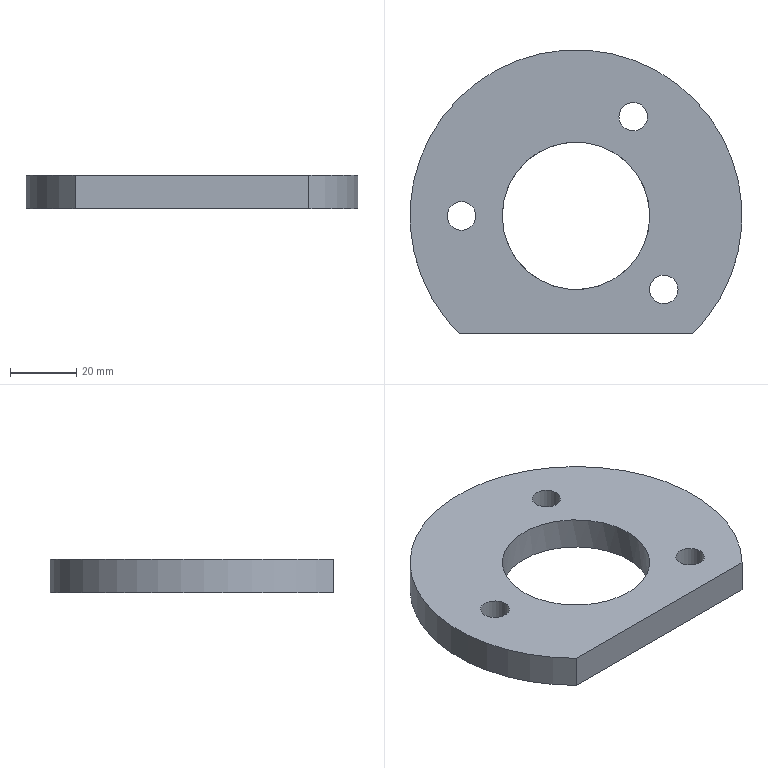Part | STEP file | 1_id802_x_t | 1 solid | 8 faces | box 100 x 85.5 x 10 mm | volume 54246 mm3 | cylinder 5 | plane 3 | commonest cylinder face diameters 8.6 x3 44.45 x1 100 x1
STEP:
#1=CARTESIAN_POINT('',(0.,0.,0.));
#2=DIRECTION('',(0.,0.,1.));
#3=DIRECTION('',(1.,0.,0.));
#4=AXIS2_PLACEMENT_3D('',#1,#2,#3);
#5=CARTESIAN_POINT('',(98.135,-31.,90.11));
#6=VERTEX_POINT('',#5);
#7=CARTESIAN_POINT('',(27.715,-31.,90.11));
#8=VERTEX_POINT('',#7);
#9=CARTESIAN_POINT('',(98.135,-31.,90.11));
#10=DIRECTION('',(-1.,0.,0.));
#11=VECTOR('',#10,1.);
#12=LINE('',#9,#11);
#13=CARTESIAN_POINT('',(62.925,4.5,90.11));
#14=DIRECTION('',(0.,0.,-1.));
#15=DIRECTION('',(-1.,0.,0.));
#16=AXIS2_PLACEMENT_3D('',#13,#14,#15);
#17=PLANE('',#16);
#18=CARTESIAN_POINT('',(-35.21,-35.5));
#19=DIRECTION('',(1.,0.));
#20=VECTOR('',#19,1.);
#21=LINE('',#18,#20);
#22=(GEOMETRIC_REPRESENTATION_CONTEXT(2)PARAMETRIC_REPRESENTATION_CONTEXT()REPRESENTATION_CONTEXT('',''));
#23=DEFINITIONAL_REPRESENTATION('',(#21),#22);
#24=PCURVE('',#17,#23);
#25=CARTESIAN_POINT('',(167.925,-31.,-58.465));
#26=DIRECTION('',(0.,1.,0.));
#27=DIRECTION('',(0.,0.,1.));
#28=AXIS2_PLACEMENT_3D('',#25,#26,#27);
#29=PLANE('',#28);
#30=CARTESIAN_POINT('',(148.575,-69.79));
#31=DIRECTION('',(0.,-1.));
#32=VECTOR('',#31,1.);
#33=LINE('',#30,#32);
#34=(GEOMETRIC_REPRESENTATION_CONTEXT(2)PARAMETRIC_REPRESENTATION_CONTEXT()REPRESENTATION_CONTEXT('',''));
#35=DEFINITIONAL_REPRESENTATION('',(#33),#34);
#36=PCURVE('',#29,#35);
#37=SURFACE_CURVE('',#12,(#24,#36),.PCURVE_S1.);
#38=EDGE_CURVE('',#6,#8,#37,.T.);
#39=ORIENTED_EDGE('',*,*,#38,.T.);
#40=CARTESIAN_POINT('',(62.925,4.5,90.11));
#41=DIRECTION('',(0.,0.,-1.));
#42=DIRECTION('',(-1.,0.,0.));
#43=AXIS2_PLACEMENT_3D('',#40,#41,#42);
#44=CIRCLE('',#43,50.);
#45=CARTESIAN_POINT('',(0.,0.));
#46=DIRECTION('',(1.,0.));
#47=AXIS2_PLACEMENT_2D('',#45,#46);
#48=CIRCLE('',#47,50.);
#49=(GEOMETRIC_REPRESENTATION_CONTEXT(2)PARAMETRIC_REPRESENTATION_CONTEXT()REPRESENTATION_CONTEXT('',''));
#50=DEFINITIONAL_REPRESENTATION('',(#48),#49);
#51=PCURVE('',#17,#50);
#52=CARTESIAN_POINT('',(62.925,4.5,100.11));
#53=DIRECTION('',(0.,0.,-1.));
#54=DIRECTION('',(-1.,0.,0.));
#55=AXIS2_PLACEMENT_3D('',#52,#53,#54);
#56=CYLINDRICAL_SURFACE('',#55,50.);
#57=CARTESIAN_POINT('',(-6.283,10.));
#58=DIRECTION('',(1.,0.));
#59=VECTOR('',#58,1.);
#60=LINE('',#57,#59);
#61=(GEOMETRIC_REPRESENTATION_CONTEXT(2)PARAMETRIC_REPRESENTATION_CONTEXT()REPRESENTATION_CONTEXT('',''));
#62=DEFINITIONAL_REPRESENTATION('',(#60),#61);
#63=PCURVE('',#56,#62);
#64=SURFACE_CURVE('',#44,(#51,#63),.PCURVE_S1.);
#65=EDGE_CURVE('',#8,#6,#64,.T.);
#66=ORIENTED_EDGE('',*,*,#65,.T.);
#67=EDGE_LOOP('',(#39,#66));
#68=FACE_BOUND('',#67,.T.);
#69=CARTESIAN_POINT('',(84.475,34.378,90.11));
#70=VERTEX_POINT('',#69);
#71=CARTESIAN_POINT('',(75.875,34.378,90.11));
#72=VERTEX_POINT('',#71);
#73=CARTESIAN_POINT('',(80.175,34.378,90.11));
#74=DIRECTION('',(0.,0.,1.));
#75=DIRECTION('',(1.,0.,0.));
#76=AXIS2_PLACEMENT_3D('',#73,#74,#75);
#77=CIRCLE('',#76,4.3);
#78=CARTESIAN_POINT('',(-21.55,29.878));
#79=CARTESIAN_POINT('',(-21.55,37.326));
#80=CARTESIAN_POINT('',(-15.1,33.602));
#81=CARTESIAN_POINT('',(-8.65,29.878));
#82=CARTESIAN_POINT('',(-15.1,26.154));
#83=CARTESIAN_POINT('',(-21.55,22.43));
#84=CARTESIAN_POINT('',(-21.55,29.878));
#85=(BOUNDED_CURVE()B_SPLINE_CURVE(2,(#78,#79,#80,#81,#82,#83,#84),.UNSPECIFIED.,.T.,.F.)B_SPLINE_CURVE_WITH_KNOTS((1,2,2,2,2,1),(-2.094,0.,2.094,4.189,6.283,8.378),.UNSPECIFIED.)CURVE()GEOMETRIC_REPRESENTATION_ITEM()RATIONAL_B_SPLINE_CURVE((1.,0.5,1.,0.5,1.,0.5,1.))REPRESENTATION_ITEM(''));
#86=(GEOMETRIC_REPRESENTATION_CONTEXT(2)PARAMETRIC_REPRESENTATION_CONTEXT()REPRESENTATION_CONTEXT('',''));
#87=DEFINITIONAL_REPRESENTATION('',(#85),#86);
#88=PCURVE('',#17,#87);
#89=CARTESIAN_POINT('',(80.175,34.378,199.11));
#90=DIRECTION('',(0.,0.,-1.));
#91=DIRECTION('',(-1.,0.,0.));
#92=AXIS2_PLACEMENT_3D('',#89,#90,#91);
#93=CYLINDRICAL_SURFACE('',#92,4.3);
#94=CARTESIAN_POINT('',(3.142,109.));
#95=DIRECTION('',(-1.,0.));
#96=VECTOR('',#95,1.);
#97=LINE('',#94,#96);
#98=(GEOMETRIC_REPRESENTATION_CONTEXT(2)PARAMETRIC_REPRESENTATION_CONTEXT()REPRESENTATION_CONTEXT('',''));
#99=DEFINITIONAL_REPRESENTATION('',(#97),#98);
#100=PCURVE('',#93,#99);
#101=SURFACE_CURVE('',#77,(#88,#100),.PCURVE_S1.);
#102=EDGE_CURVE('',#70,#72,#101,.T.);
#103=ORIENTED_EDGE('',*,*,#102,.T.);
#104=CARTESIAN_POINT('',(80.175,34.378,90.11));
#105=DIRECTION('',(0.,0.,1.));
#106=DIRECTION('',(1.,0.,0.));
#107=AXIS2_PLACEMENT_3D('',#104,#105,#106);
#108=CIRCLE('',#107,4.3);
#109=CARTESIAN_POINT('',(-21.55,29.878));
#110=CARTESIAN_POINT('',(-21.55,37.326));
#111=CARTESIAN_POINT('',(-15.1,33.602));
#112=CARTESIAN_POINT('',(-8.65,29.878));
#113=CARTESIAN_POINT('',(-15.1,26.154));
#114=CARTESIAN_POINT('',(-21.55,22.43));
#115=CARTESIAN_POINT('',(-21.55,29.878));
#116=(BOUNDED_CURVE()B_SPLINE_CURVE(2,(#109,#110,#111,#112,#113,#114,#115),.UNSPECIFIED.,.T.,.F.)B_SPLINE_CURVE_WITH_KNOTS((1,2,2,2,2,1),(-2.094,0.,2.094,4.189,6.283,8.378),.UNSPECIFIED.)CURVE()GEOMETRIC_REPRESENTATION_ITEM()RATIONAL_B_SPLINE_CURVE((1.,0.5,1.,0.5,1.,0.5,1.))REPRESENTATION_ITEM(''));
#117=(GEOMETRIC_REPRESENTATION_CONTEXT(2)PARAMETRIC_REPRESENTATION_CONTEXT()REPRESENTATION_CONTEXT('',''));
#118=DEFINITIONAL_REPRESENTATION('',(#116),#117);
#119=PCURVE('',#17,#118);
#120=CARTESIAN_POINT('',(9.425,109.));
#121=DIRECTION('',(-1.,0.));
#122=VECTOR('',#121,1.);
#123=LINE('',#120,#122);
#124=(GEOMETRIC_REPRESENTATION_CONTEXT(2)PARAMETRIC_REPRESENTATION_CONTEXT()REPRESENTATION_CONTEXT('',''));
#125=DEFINITIONAL_REPRESENTATION('',(#123),#124);
#126=PCURVE('',#93,#125);
#127=SURFACE_CURVE('',#108,(#119,#126),.PCURVE_S1.);
#128=EDGE_CURVE('',#72,#70,#127,.T.);
#129=ORIENTED_EDGE('',*,*,#128,.T.);
#130=EDGE_LOOP('',(#103,#129));
#131=FACE_BOUND('',#130,.T.);
#132=CARTESIAN_POINT('',(32.725,4.5,90.11));
#133=VERTEX_POINT('',#132);
#134=CARTESIAN_POINT('',(28.425,4.5,90.11));
#135=DIRECTION('',(0.,0.,1.));
#136=DIRECTION('',(1.,0.,0.));
#137=AXIS2_PLACEMENT_3D('',#134,#135,#136);
#138=CIRCLE('',#137,4.3);
#139=CARTESIAN_POINT('',(30.2,0.));
#140=CARTESIAN_POINT('',(30.2,7.448));
#141=CARTESIAN_POINT('',(36.65,3.724));
#142=CARTESIAN_POINT('',(43.1,0.));
#143=CARTESIAN_POINT('',(36.65,-3.724));
#144=CARTESIAN_POINT('',(30.2,-7.448));
#145=CARTESIAN_POINT('',(30.2,0.));
#146=(BOUNDED_CURVE()B_SPLINE_CURVE(2,(#139,#140,#141,#142,#143,#144,#145),.UNSPECIFIED.,.T.,.F.)B_SPLINE_CURVE_WITH_KNOTS((1,2,2,2,2,1),(-2.094,0.,2.094,4.189,6.283,8.378),.UNSPECIFIED.)CURVE()GEOMETRIC_REPRESENTATION_ITEM()RATIONAL_B_SPLINE_CURVE((1.,0.5,1.,0.5,1.,0.5,1.))REPRESENTATION_ITEM(''));
#147=(GEOMETRIC_REPRESENTATION_CONTEXT(2)PARAMETRIC_REPRESENTATION_CONTEXT()REPRESENTATION_CONTEXT('',''));
#148=DEFINITIONAL_REPRESENTATION('',(#146),#147);
#149=PCURVE('',#17,#148);
#150=CARTESIAN_POINT('',(28.425,4.5,199.11));
#151=DIRECTION('',(0.,0.,-1.));
#152=DIRECTION('',(-1.,0.,0.));
#153=AXIS2_PLACEMENT_3D('',#150,#151,#152);
#154=CYLINDRICAL_SURFACE('',#153,4.3);
#155=CARTESIAN_POINT('',(9.425,109.));
#156=DIRECTION('',(-1.,0.));
#157=VECTOR('',#156,1.);
#158=LINE('',#155,#157);
#159=(GEOMETRIC_REPRESENTATION_CONTEXT(2)PARAMETRIC_REPRESENTATION_CONTEXT()REPRESENTATION_CONTEXT('',''));
#160=DEFINITIONAL_REPRESENTATION('',(#158),#159);
#161=PCURVE('',#154,#160);
#162=SURFACE_CURVE('',#138,(#149,#161),.PCURVE_S1.);
#163=EDGE_CURVE('',#133,#133,#162,.T.);
#164=ORIENTED_EDGE('',*,*,#163,.T.);
#165=EDGE_LOOP('',(#164));
#166=FACE_BOUND('',#165,.T.);
#167=CARTESIAN_POINT('',(93.654,-17.676,90.11));
#168=VERTEX_POINT('',#167);
#169=CARTESIAN_POINT('',(89.354,-17.676,90.11));
#170=DIRECTION('',(0.,0.,1.));
#171=DIRECTION('',(1.,0.,0.));
#172=AXIS2_PLACEMENT_3D('',#169,#170,#171);
#173=CIRCLE('',#172,4.3);
#174=CARTESIAN_POINT('',(-30.729,-22.176));
#175=CARTESIAN_POINT('',(-30.729,-14.728));
#176=CARTESIAN_POINT('',(-24.279,-18.452));
#177=CARTESIAN_POINT('',(-17.829,-22.176));
#178=CARTESIAN_POINT('',(-24.279,-25.9));
#179=CARTESIAN_POINT('',(-30.729,-29.624));
#180=CARTESIAN_POINT('',(-30.729,-22.176));
#181=(BOUNDED_CURVE()B_SPLINE_CURVE(2,(#174,#175,#176,#177,#178,#179,#180),.UNSPECIFIED.,.T.,.F.)B_SPLINE_CURVE_WITH_KNOTS((1,2,2,2,2,1),(-2.094,0.,2.094,4.189,6.283,8.378),.UNSPECIFIED.)CURVE()GEOMETRIC_REPRESENTATION_ITEM()RATIONAL_B_SPLINE_CURVE((1.,0.5,1.,0.5,1.,0.5,1.))REPRESENTATION_ITEM(''));
#182=(GEOMETRIC_REPRESENTATION_CONTEXT(2)PARAMETRIC_REPRESENTATION_CONTEXT()REPRESENTATION_CONTEXT('',''));
#183=DEFINITIONAL_REPRESENTATION('',(#181),#182);
#184=PCURVE('',#17,#183);
#185=CARTESIAN_POINT('',(89.354,-17.676,199.11));
#186=DIRECTION('',(0.,0.,-1.));
#187=DIRECTION('',(-1.,0.,0.));
#188=AXIS2_PLACEMENT_3D('',#185,#186,#187);
#189=CYLINDRICAL_SURFACE('',#188,4.3);
#190=CARTESIAN_POINT('',(9.425,109.));
#191=DIRECTION('',(-1.,0.));
#192=VECTOR('',#191,1.);
#193=LINE('',#190,#192);
#194=(GEOMETRIC_REPRESENTATION_CONTEXT(2)PARAMETRIC_REPRESENTATION_CONTEXT()REPRESENTATION_CONTEXT('',''));
#195=DEFINITIONAL_REPRESENTATION('',(#193),#194);
#196=PCURVE('',#189,#195);
#197=SURFACE_CURVE('',#173,(#184,#196),.PCURVE_S1.);
#198=EDGE_CURVE('',#168,#168,#197,.T.);
#199=ORIENTED_EDGE('',*,*,#198,.T.);
#200=EDGE_LOOP('',(#199));
#201=FACE_BOUND('',#200,.T.);
#202=CARTESIAN_POINT('',(40.7,4.5,90.11));
#203=VERTEX_POINT('',#202);
#204=CARTESIAN_POINT('',(62.925,4.5,90.11));
#205=DIRECTION('',(0.,0.,1.));
#206=DIRECTION('',(-1.,0.,0.));
#207=AXIS2_PLACEMENT_3D('',#204,#205,#206);
#208=CIRCLE('',#207,22.225);
#209=CARTESIAN_POINT('',(22.225,0.));
#210=CARTESIAN_POINT('',(22.225,-38.495));
#211=CARTESIAN_POINT('',(-11.113,-19.247));
#212=CARTESIAN_POINT('',(-44.45,0.));
#213=CARTESIAN_POINT('',(-11.113,19.247));
#214=CARTESIAN_POINT('',(22.225,38.495));
#215=CARTESIAN_POINT('',(22.225,0.));
#216=(BOUNDED_CURVE()B_SPLINE_CURVE(2,(#209,#210,#211,#212,#213,#214,#215),.UNSPECIFIED.,.T.,.F.)B_SPLINE_CURVE_WITH_KNOTS((1,2,2,2,2,1),(-2.094,0.,2.094,4.189,6.283,8.378),.UNSPECIFIED.)CURVE()GEOMETRIC_REPRESENTATION_ITEM()RATIONAL_B_SPLINE_CURVE((1.,0.5,1.,0.5,1.,0.5,1.))REPRESENTATION_ITEM(''));
#217=(GEOMETRIC_REPRESENTATION_CONTEXT(2)PARAMETRIC_REPRESENTATION_CONTEXT()REPRESENTATION_CONTEXT('',''));
#218=DEFINITIONAL_REPRESENTATION('',(#216),#217);
#219=PCURVE('',#17,#218);
#220=CARTESIAN_POINT('',(62.925,4.5,91.735));
#221=DIRECTION('',(0.,0.,1.));
#222=DIRECTION('',(-0.5,0.866,0.));
#223=AXIS2_PLACEMENT_3D('',#220,#221,#222);
#224=CYLINDRICAL_SURFACE('',#223,22.225);
#225=CARTESIAN_POINT('',(1.047,-1.625));
#226=DIRECTION('',(1.,0.));
#227=VECTOR('',#226,1.);
#228=LINE('',#225,#227);
#229=(GEOMETRIC_REPRESENTATION_CONTEXT(2)PARAMETRIC_REPRESENTATION_CONTEXT()REPRESENTATION_CONTEXT('',''));
#230=DEFINITIONAL_REPRESENTATION('',(#228),#229);
#231=PCURVE('',#224,#230);
#232=SURFACE_CURVE('',#208,(#219,#231),.PCURVE_S1.);
#233=EDGE_CURVE('',#203,#203,#232,.T.);
#234=ORIENTED_EDGE('',*,*,#233,.T.);
#235=EDGE_LOOP('',(#234));
#236=FACE_BOUND('',#235,.T.);
#237=ADVANCED_FACE('',(#68,#131,#166,#201,#236),#17,.T.);
#238=ORIENTED_EDGE('',*,*,#102,.T.);
#239=CARTESIAN_POINT('',(75.875,34.378,100.11));
#240=VERTEX_POINT('',#239);
#241=CARTESIAN_POINT('',(75.875,34.378,100.11));
#242=CARTESIAN_POINT('',(75.875,34.378,90.11));
#243=B_SPLINE_CURVE_WITH_KNOTS('',1,(#241,#242),.UNSPECIFIED.,.F.,.F.,(2,2),(99.,109.),.PIECEWISE_BEZIER_KNOTS.);
#244=CARTESIAN_POINT('',(0.,0.));
#245=DIRECTION('',(0.,1.));
#246=VECTOR('',#245,1.);
#247=LINE('',#244,#246);
#248=(GEOMETRIC_REPRESENTATION_CONTEXT(2)PARAMETRIC_REPRESENTATION_CONTEXT()REPRESENTATION_CONTEXT('',''));
#249=DEFINITIONAL_REPRESENTATION('',(#247),#248);
#250=PCURVE('',#93,#249);
#251=CARTESIAN_POINT('',(6.283,0.));
#252=DIRECTION('',(0.,1.));
#253=VECTOR('',#252,1.);
#254=LINE('',#251,#253);
#255=(GEOMETRIC_REPRESENTATION_CONTEXT(2)PARAMETRIC_REPRESENTATION_CONTEXT()REPRESENTATION_CONTEXT('',''));
#256=DEFINITIONAL_REPRESENTATION('',(#254),#255);
#257=PCURVE('',#93,#256);
#258=SEAM_CURVE('',#243,(#250,#257),.PCURVE_S1.);
#259=EDGE_CURVE('',#240,#72,#258,.T.);
#260=ORIENTED_EDGE('',*,*,#259,.F.);
#261=CARTESIAN_POINT('',(80.175,34.378,100.11));
#262=DIRECTION('',(0.,0.,-1.));
#263=DIRECTION('',(-1.,0.,0.));
#264=AXIS2_PLACEMENT_3D('',#261,#262,#263);
#265=CIRCLE('',#264,4.3);
#266=CARTESIAN_POINT('',(0.,99.));
#267=DIRECTION('',(1.,0.));
#268=VECTOR('',#267,1.);
#269=LINE('',#266,#268);
#270=(GEOMETRIC_REPRESENTATION_CONTEXT(2)PARAMETRIC_REPRESENTATION_CONTEXT()REPRESENTATION_CONTEXT('',''));
#271=DEFINITIONAL_REPRESENTATION('',(#269),#270);
#272=PCURVE('',#93,#271);
#273=CARTESIAN_POINT('',(62.925,4.5,100.11));
#274=DIRECTION('',(0.,0.,-1.));
#275=DIRECTION('',(-1.,0.,0.));
#276=AXIS2_PLACEMENT_3D('',#273,#274,#275);
#277=PLANE('',#276);
#278=CARTESIAN_POINT('',(-17.25,29.878));
#279=DIRECTION('',(1.,0.));
#280=AXIS2_PLACEMENT_2D('',#278,#279);
#281=CIRCLE('',#280,4.3);
#282=(GEOMETRIC_REPRESENTATION_CONTEXT(2)PARAMETRIC_REPRESENTATION_CONTEXT()REPRESENTATION_CONTEXT('',''));
#283=DEFINITIONAL_REPRESENTATION('',(#281),#282);
#284=PCURVE('',#277,#283);
#285=SURFACE_CURVE('',#265,(#272,#284),.PCURVE_S1.);
#286=EDGE_CURVE('',#240,#240,#285,.T.);
#287=ORIENTED_EDGE('',*,*,#286,.T.);
#288=ORIENTED_EDGE('',*,*,#259,.T.);
#289=ORIENTED_EDGE('',*,*,#128,.T.);
#290=EDGE_LOOP('',(#238,#260,#287,#288,#289));
#291=FACE_BOUND('',#290,.F.);
#292=ADVANCED_FACE('',(#291),#93,.F.);
#293=CARTESIAN_POINT('',(98.135,-31.,100.11));
#294=VERTEX_POINT('',#293);
#295=CARTESIAN_POINT('',(27.715,-31.,100.11));
#296=VERTEX_POINT('',#295);
#297=CARTESIAN_POINT('',(62.925,4.5,100.11));
#298=DIRECTION('',(0.,0.,1.));
#299=DIRECTION('',(0.7042,-0.71,0.));
#300=AXIS2_PLACEMENT_3D('',#297,#298,#299);
#301=CIRCLE('',#300,50.);
#302=CARTESIAN_POINT('',(-35.21,-35.5));
#303=CARTESIAN_POINT('',(-96.698,25.486));
#304=CARTESIAN_POINT('',(-13.139,48.243));
#305=CARTESIAN_POINT('',(70.42,71.));
#306=CARTESIAN_POINT('',(48.349,-12.743));
#307=CARTESIAN_POINT('',(26.278,-96.486));
#308=CARTESIAN_POINT('',(-35.21,-35.5));
#309=(BOUNDED_CURVE()B_SPLINE_CURVE(2,(#302,#303,#304,#305,#306,#307,#308),.UNSPECIFIED.,.T.,.F.)B_SPLINE_CURVE_WITH_KNOTS((1,2,2,2,2,1),(-2.094,0.,2.094,4.189,6.283,8.378),.UNSPECIFIED.)CURVE()GEOMETRIC_REPRESENTATION_ITEM()RATIONAL_B_SPLINE_CURVE((1.,0.5,1.,0.5,1.,0.5,1.))REPRESENTATION_ITEM(''));
#310=(GEOMETRIC_REPRESENTATION_CONTEXT(2)PARAMETRIC_REPRESENTATION_CONTEXT()REPRESENTATION_CONTEXT('',''));
#311=DEFINITIONAL_REPRESENTATION('',(#309),#310);
#312=PCURVE('',#277,#311);
#313=CARTESIAN_POINT('',(3.931,0.));
#314=DIRECTION('',(-1.,0.));
#315=VECTOR('',#314,1.);
#316=LINE('',#313,#315);
#317=(GEOMETRIC_REPRESENTATION_CONTEXT(2)PARAMETRIC_REPRESENTATION_CONTEXT()REPRESENTATION_CONTEXT('',''));
#318=DEFINITIONAL_REPRESENTATION('',(#316),#317);
#319=PCURVE('',#56,#318);
#320=SURFACE_CURVE('',#301,(#312,#319),.PCURVE_S1.);
#321=EDGE_CURVE('',#294,#296,#320,.T.);
#322=ORIENTED_EDGE('',*,*,#321,.T.);
#323=CARTESIAN_POINT('',(98.135,-31.,100.11));
#324=DIRECTION('',(-1.,0.,0.));
#325=VECTOR('',#324,1.);
#326=LINE('',#323,#325);
#327=CARTESIAN_POINT('',(-35.21,-35.5));
#328=DIRECTION('',(1.,0.));
#329=VECTOR('',#328,1.);
#330=LINE('',#327,#329);
#331=(GEOMETRIC_REPRESENTATION_CONTEXT(2)PARAMETRIC_REPRESENTATION_CONTEXT()REPRESENTATION_CONTEXT('',''));
#332=DEFINITIONAL_REPRESENTATION('',(#330),#331);
#333=PCURVE('',#277,#332);
#334=CARTESIAN_POINT('',(158.575,-69.79));
#335=DIRECTION('',(0.,-1.));
#336=VECTOR('',#335,1.);
#337=LINE('',#334,#336);
#338=(GEOMETRIC_REPRESENTATION_CONTEXT(2)PARAMETRIC_REPRESENTATION_CONTEXT()REPRESENTATION_CONTEXT('',''));
#339=DEFINITIONAL_REPRESENTATION('',(#337),#338);
#340=PCURVE('',#29,#339);
#341=SURFACE_CURVE('',#326,(#333,#340),.PCURVE_S1.);
#342=EDGE_CURVE('',#294,#296,#341,.T.);
#343=ORIENTED_EDGE('',*,*,#342,.F.);
#344=EDGE_LOOP('',(#322,#343));
#345=FACE_BOUND('',#344,.T.);
#346=ORIENTED_EDGE('',*,*,#286,.T.);
#347=EDGE_LOOP('',(#346));
#348=FACE_BOUND('',#347,.T.);
#349=CARTESIAN_POINT('',(32.725,4.5,100.11));
#350=VERTEX_POINT('',#349);
#351=CARTESIAN_POINT('',(28.425,4.5,100.11));
#352=DIRECTION('',(0.,0.,-1.));
#353=DIRECTION('',(1.,0.,0.));
#354=AXIS2_PLACEMENT_3D('',#351,#352,#353);
#355=CIRCLE('',#354,4.3);
#356=CARTESIAN_POINT('',(34.5,0.));
#357=DIRECTION('',(-1.,0.));
#358=AXIS2_PLACEMENT_2D('',#356,#357);
#359=CIRCLE('',#358,4.3);
#360=(GEOMETRIC_REPRESENTATION_CONTEXT(2)PARAMETRIC_REPRESENTATION_CONTEXT()REPRESENTATION_CONTEXT('',''));
#361=DEFINITIONAL_REPRESENTATION('',(#359),#360);
#362=PCURVE('',#277,#361);
#363=CARTESIAN_POINT('',(3.142,99.));
#364=DIRECTION('',(1.,0.));
#365=VECTOR('',#364,1.);
#366=LINE('',#363,#365);
#367=(GEOMETRIC_REPRESENTATION_CONTEXT(2)PARAMETRIC_REPRESENTATION_CONTEXT()REPRESENTATION_CONTEXT('',''));
#368=DEFINITIONAL_REPRESENTATION('',(#366),#367);
#369=PCURVE('',#154,#368);
#370=SURFACE_CURVE('',#355,(#362,#369),.PCURVE_S1.);
#371=EDGE_CURVE('',#350,#350,#370,.T.);
#372=ORIENTED_EDGE('',*,*,#371,.T.);
#373=EDGE_LOOP('',(#372));
#374=FACE_BOUND('',#373,.T.);
#375=CARTESIAN_POINT('',(93.654,-17.676,100.11));
#376=VERTEX_POINT('',#375);
#377=CARTESIAN_POINT('',(89.354,-17.676,100.11));
#378=DIRECTION('',(0.,0.,-1.));
#379=DIRECTION('',(1.,0.,0.));
#380=AXIS2_PLACEMENT_3D('',#377,#378,#379);
#381=CIRCLE('',#380,4.3);
#382=CARTESIAN_POINT('',(-26.429,-22.176));
#383=DIRECTION('',(-1.,0.));
#384=AXIS2_PLACEMENT_2D('',#382,#383);
#385=CIRCLE('',#384,4.3);
#386=(GEOMETRIC_REPRESENTATION_CONTEXT(2)PARAMETRIC_REPRESENTATION_CONTEXT()REPRESENTATION_CONTEXT('',''));
#387=DEFINITIONAL_REPRESENTATION('',(#385),#386);
#388=PCURVE('',#277,#387);
#389=CARTESIAN_POINT('',(3.142,99.));
#390=DIRECTION('',(1.,0.));
#391=VECTOR('',#390,1.);
#392=LINE('',#389,#391);
#393=(GEOMETRIC_REPRESENTATION_CONTEXT(2)PARAMETRIC_REPRESENTATION_CONTEXT()REPRESENTATION_CONTEXT('',''));
#394=DEFINITIONAL_REPRESENTATION('',(#392),#393);
#395=PCURVE('',#189,#394);
#396=SURFACE_CURVE('',#381,(#388,#395),.PCURVE_S1.);
#397=EDGE_CURVE('',#376,#376,#396,.T.);
#398=ORIENTED_EDGE('',*,*,#397,.T.);
#399=EDGE_LOOP('',(#398));
#400=FACE_BOUND('',#399,.T.);
#401=CARTESIAN_POINT('',(85.15,4.5,100.11));
#402=VERTEX_POINT('',#401);
#403=CARTESIAN_POINT('',(40.7,4.5,100.11));
#404=VERTEX_POINT('',#403);
#405=CARTESIAN_POINT('',(62.925,4.5,100.11));
#406=DIRECTION('',(0.,0.,-1.));
#407=DIRECTION('',(1.,0.,0.));
#408=AXIS2_PLACEMENT_3D('',#405,#406,#407);
#409=CIRCLE('',#408,22.225);
#410=CARTESIAN_POINT('',(0.,0.));
#411=DIRECTION('',(-1.,0.));
#412=AXIS2_PLACEMENT_2D('',#410,#411);
#413=CIRCLE('',#412,22.225);
#414=(GEOMETRIC_REPRESENTATION_CONTEXT(2)PARAMETRIC_REPRESENTATION_CONTEXT()REPRESENTATION_CONTEXT('',''));
#415=DEFINITIONAL_REPRESENTATION('',(#413),#414);
#416=PCURVE('',#277,#415);
#417=CARTESIAN_POINT('',(4.189,8.375));
#418=DIRECTION('',(-1.,0.));
#419=VECTOR('',#418,1.);
#420=LINE('',#417,#419);
#421=(GEOMETRIC_REPRESENTATION_CONTEXT(2)PARAMETRIC_REPRESENTATION_CONTEXT()REPRESENTATION_CONTEXT('',''));
#422=DEFINITIONAL_REPRESENTATION('',(#420),#421);
#423=PCURVE('',#224,#422);
#424=SURFACE_CURVE('',#409,(#416,#423),.PCURVE_S1.);
#425=EDGE_CURVE('',#402,#404,#424,.T.);
#426=ORIENTED_EDGE('',*,*,#425,.T.);
#427=CARTESIAN_POINT('',(62.925,4.5,100.11));
#428=DIRECTION('',(0.,0.,-1.));
#429=DIRECTION('',(1.,0.,0.));
#430=AXIS2_PLACEMENT_3D('',#427,#428,#429);
#431=CIRCLE('',#430,22.225);
#432=CARTESIAN_POINT('',(0.,0.));
#433=DIRECTION('',(-1.,0.));
#434=AXIS2_PLACEMENT_2D('',#432,#433);
#435=CIRCLE('',#434,22.225);
#436=(GEOMETRIC_REPRESENTATION_CONTEXT(2)PARAMETRIC_REPRESENTATION_CONTEXT()REPRESENTATION_CONTEXT('',''));
#437=DEFINITIONAL_REPRESENTATION('',(#435),#436);
#438=PCURVE('',#277,#437);
#439=CARTESIAN_POINT('',(10.472,8.375));
#440=DIRECTION('',(-1.,0.));
#441=VECTOR('',#440,1.);
#442=LINE('',#439,#441);
#443=(GEOMETRIC_REPRESENTATION_CONTEXT(2)PARAMETRIC_REPRESENTATION_CONTEXT()REPRESENTATION_CONTEXT('',''));
#444=DEFINITIONAL_REPRESENTATION('',(#442),#443);
#445=PCURVE('',#224,#444);
#446=SURFACE_CURVE('',#431,(#438,#445),.PCURVE_S1.);
#447=EDGE_CURVE('',#404,#402,#446,.T.);
#448=ORIENTED_EDGE('',*,*,#447,.T.);
#449=EDGE_LOOP('',(#426,#448));
#450=FACE_BOUND('',#449,.T.);
#451=ADVANCED_FACE('',(#345,#348,#374,#400,#450),#277,.F.);
#452=ORIENTED_EDGE('',*,*,#163,.T.);
#453=CARTESIAN_POINT('',(32.725,4.5,100.11));
#454=CARTESIAN_POINT('',(32.725,4.5,90.11));
#455=B_SPLINE_CURVE_WITH_KNOTS('',1,(#453,#454),.UNSPECIFIED.,.F.,.F.,(2,2),(99.,109.),.PIECEWISE_BEZIER_KNOTS.);
#456=CARTESIAN_POINT('',(3.142,0.));
#457=DIRECTION('',(0.,1.));
#458=VECTOR('',#457,1.);
#459=LINE('',#456,#458);
#460=(GEOMETRIC_REPRESENTATION_CONTEXT(2)PARAMETRIC_REPRESENTATION_CONTEXT()REPRESENTATION_CONTEXT('',''));
#461=DEFINITIONAL_REPRESENTATION('',(#459),#460);
#462=PCURVE('',#154,#461);
#463=CARTESIAN_POINT('',(9.425,0.));
#464=DIRECTION('',(0.,1.));
#465=VECTOR('',#464,1.);
#466=LINE('',#463,#465);
#467=(GEOMETRIC_REPRESENTATION_CONTEXT(2)PARAMETRIC_REPRESENTATION_CONTEXT()REPRESENTATION_CONTEXT('',''));
#468=DEFINITIONAL_REPRESENTATION('',(#466),#467);
#469=PCURVE('',#154,#468);
#470=SEAM_CURVE('',#455,(#462,#469),.PCURVE_S1.);
#471=EDGE_CURVE('',#350,#133,#470,.T.);
#472=ORIENTED_EDGE('',*,*,#471,.F.);
#473=ORIENTED_EDGE('',*,*,#371,.T.);
#474=ORIENTED_EDGE('',*,*,#471,.T.);
#475=EDGE_LOOP('',(#452,#472,#473,#474));
#476=FACE_BOUND('',#475,.F.);
#477=ADVANCED_FACE('',(#476),#154,.F.);
#478=ORIENTED_EDGE('',*,*,#198,.T.);
#479=CARTESIAN_POINT('',(93.654,-17.676,100.11));
#480=CARTESIAN_POINT('',(93.654,-17.676,90.11));
#481=B_SPLINE_CURVE_WITH_KNOTS('',1,(#479,#480),.UNSPECIFIED.,.F.,.F.,(2,2),(99.,109.),.PIECEWISE_BEZIER_KNOTS.);
#482=CARTESIAN_POINT('',(3.142,0.));
#483=DIRECTION('',(0.,1.));
#484=VECTOR('',#483,1.);
#485=LINE('',#482,#484);
#486=(GEOMETRIC_REPRESENTATION_CONTEXT(2)PARAMETRIC_REPRESENTATION_CONTEXT()REPRESENTATION_CONTEXT('',''));
#487=DEFINITIONAL_REPRESENTATION('',(#485),#486);
#488=PCURVE('',#189,#487);
#489=CARTESIAN_POINT('',(9.425,0.));
#490=DIRECTION('',(0.,1.));
#491=VECTOR('',#490,1.);
#492=LINE('',#489,#491);
#493=(GEOMETRIC_REPRESENTATION_CONTEXT(2)PARAMETRIC_REPRESENTATION_CONTEXT()REPRESENTATION_CONTEXT('',''));
#494=DEFINITIONAL_REPRESENTATION('',(#492),#493);
#495=PCURVE('',#189,#494);
#496=SEAM_CURVE('',#481,(#488,#495),.PCURVE_S1.);
#497=EDGE_CURVE('',#376,#168,#496,.T.);
#498=ORIENTED_EDGE('',*,*,#497,.F.);
#499=ORIENTED_EDGE('',*,*,#397,.T.);
#500=ORIENTED_EDGE('',*,*,#497,.T.);
#501=EDGE_LOOP('',(#478,#498,#499,#500));
#502=FACE_BOUND('',#501,.F.);
#503=ADVANCED_FACE('',(#502),#189,.F.);
#504=ORIENTED_EDGE('',*,*,#425,.T.);
#505=CARTESIAN_POINT('',(40.7,4.5,90.11));
#506=CARTESIAN_POINT('',(40.7,4.5,100.11));
#507=B_SPLINE_CURVE_WITH_KNOTS('',1,(#505,#506),.UNSPECIFIED.,.F.,.F.,(2,2),(-1.625,8.375),.PIECEWISE_BEZIER_KNOTS.);
#508=CARTESIAN_POINT('',(1.047,0.));
#509=DIRECTION('',(0.,1.));
#510=VECTOR('',#509,1.);
#511=LINE('',#508,#510);
#512=(GEOMETRIC_REPRESENTATION_CONTEXT(2)PARAMETRIC_REPRESENTATION_CONTEXT()REPRESENTATION_CONTEXT('',''));
#513=DEFINITIONAL_REPRESENTATION('',(#511),#512);
#514=PCURVE('',#224,#513);
#515=CARTESIAN_POINT('',(7.33,0.));
#516=DIRECTION('',(0.,1.));
#517=VECTOR('',#516,1.);
#518=LINE('',#515,#517);
#519=(GEOMETRIC_REPRESENTATION_CONTEXT(2)PARAMETRIC_REPRESENTATION_CONTEXT()REPRESENTATION_CONTEXT('',''));
#520=DEFINITIONAL_REPRESENTATION('',(#518),#519);
#521=PCURVE('',#224,#520);
#522=SEAM_CURVE('',#507,(#514,#521),.PCURVE_S1.);
#523=EDGE_CURVE('',#203,#404,#522,.T.);
#524=ORIENTED_EDGE('',*,*,#523,.F.);
#525=ORIENTED_EDGE('',*,*,#233,.T.);
#526=ORIENTED_EDGE('',*,*,#523,.T.);
#527=ORIENTED_EDGE('',*,*,#447,.T.);
#528=EDGE_LOOP('',(#504,#524,#525,#526,#527));
#529=FACE_BOUND('',#528,.F.);
#530=ADVANCED_FACE('',(#529),#224,.F.);
#531=ORIENTED_EDGE('',*,*,#65,.F.);
#532=CARTESIAN_POINT('',(27.715,-31.,90.11));
#533=DIRECTION('',(0.,0.,1.));
#534=VECTOR('',#533,1.);
#535=LINE('',#532,#534);
#536=CARTESIAN_POINT('',(-0.7895,10.));
#537=DIRECTION('',(0.,-1.));
#538=VECTOR('',#537,1.);
#539=LINE('',#536,#538);
#540=(GEOMETRIC_REPRESENTATION_CONTEXT(2)PARAMETRIC_REPRESENTATION_CONTEXT()REPRESENTATION_CONTEXT('',''));
#541=DEFINITIONAL_REPRESENTATION('',(#539),#540);
#542=PCURVE('',#56,#541);
#543=CARTESIAN_POINT('',(148.575,-140.21));
#544=DIRECTION('',(1.,0.));
#545=VECTOR('',#544,1.);
#546=LINE('',#543,#545);
#547=(GEOMETRIC_REPRESENTATION_CONTEXT(2)PARAMETRIC_REPRESENTATION_CONTEXT()REPRESENTATION_CONTEXT('',''));
#548=DEFINITIONAL_REPRESENTATION('',(#546),#547);
#549=PCURVE('',#29,#548);
#550=SURFACE_CURVE('',#535,(#542,#549),.PCURVE_S1.);
#551=EDGE_CURVE('',#8,#296,#550,.T.);
#552=ORIENTED_EDGE('',*,*,#551,.T.);
#553=ORIENTED_EDGE('',*,*,#321,.F.);
#554=CARTESIAN_POINT('',(98.135,-31.,100.11));
#555=DIRECTION('',(0.,0.,-1.));
#556=VECTOR('',#555,1.);
#557=LINE('',#554,#556);
#558=CARTESIAN_POINT('',(3.931,0.));
#559=DIRECTION('',(0.,1.));
#560=VECTOR('',#559,1.);
#561=LINE('',#558,#560);
#562=(GEOMETRIC_REPRESENTATION_CONTEXT(2)PARAMETRIC_REPRESENTATION_CONTEXT()REPRESENTATION_CONTEXT('',''));
#563=DEFINITIONAL_REPRESENTATION('',(#561),#562);
#564=PCURVE('',#56,#563);
#565=CARTESIAN_POINT('',(158.575,-69.79));
#566=DIRECTION('',(-1.,0.));
#567=VECTOR('',#566,1.);
#568=LINE('',#565,#567);
#569=(GEOMETRIC_REPRESENTATION_CONTEXT(2)PARAMETRIC_REPRESENTATION_CONTEXT()REPRESENTATION_CONTEXT('',''));
#570=DEFINITIONAL_REPRESENTATION('',(#568),#569);
#571=PCURVE('',#29,#570);
#572=SURFACE_CURVE('',#557,(#564,#571),.PCURVE_S1.);
#573=EDGE_CURVE('',#294,#6,#572,.T.);
#574=ORIENTED_EDGE('',*,*,#573,.T.);
#575=EDGE_LOOP('',(#531,#552,#553,#574));
#576=FACE_BOUND('',#575,.T.);
#577=ADVANCED_FACE('',(#576),#56,.T.);
#578=ORIENTED_EDGE('',*,*,#573,.F.);
#579=ORIENTED_EDGE('',*,*,#342,.T.);
#580=ORIENTED_EDGE('',*,*,#551,.F.);
#581=ORIENTED_EDGE('',*,*,#38,.F.);
#582=EDGE_LOOP('',(#578,#579,#580,#581));
#583=FACE_BOUND('',#582,.T.);
#584=ADVANCED_FACE('',(#583),#29,.F.);
#585=CLOSED_SHELL('',(#237,#292,#451,#477,#503,#530,#577,#584));
#586=MANIFOLD_SOLID_BREP('',#585);
#587=(LENGTH_UNIT()NAMED_UNIT(*)SI_UNIT(.MILLI.,.METRE.));
#588=UNCERTAINTY_MEASURE_WITH_UNIT(LENGTH_MEASURE(0.000005),#587,'','');
#589=(NAMED_UNIT(*)PLANE_ANGLE_UNIT()SI_UNIT($,.RADIAN.));
#590=(NAMED_UNIT(*)SI_UNIT($,.STERADIAN.)SOLID_ANGLE_UNIT());
#591=(GEOMETRIC_REPRESENTATION_CONTEXT(3)GLOBAL_UNCERTAINTY_ASSIGNED_CONTEXT((#588))GLOBAL_UNIT_ASSIGNED_CONTEXT((#587,#589,#590))REPRESENTATION_CONTEXT('',''));
#592=ADVANCED_BREP_SHAPE_REPRESENTATION('',(#4,#586),#591);